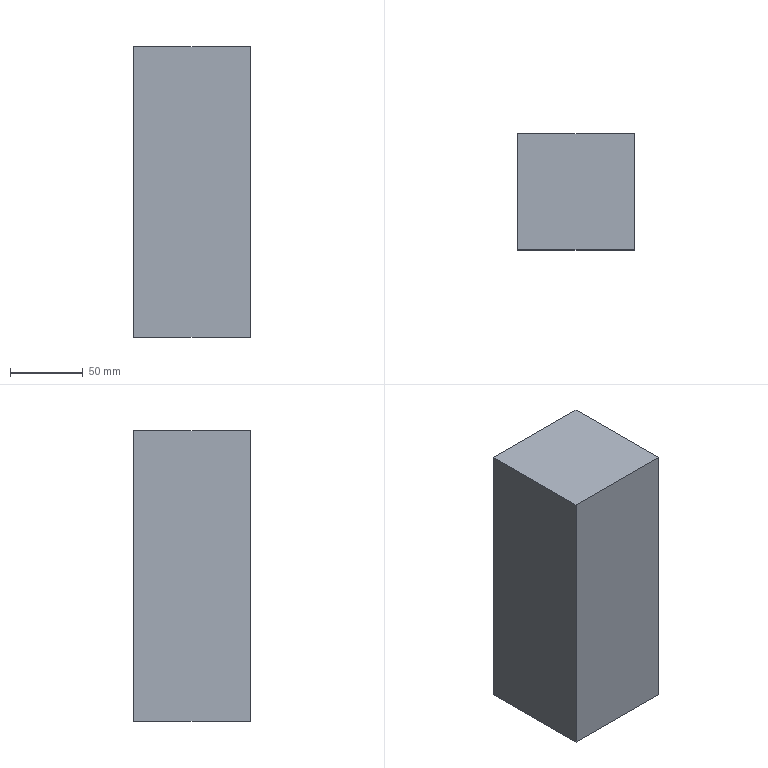Part | SolidWorks | features Extrusion 1 | 1 solid | 6 faces | box 80 x 80 x 200 mm | volume 1280000 mm3 | plane 6
STEP:
#1=CARTESIAN_POINT('',(40.,-40.,-100.));
#2=VERTEX_POINT('',#1);
#3=CARTESIAN_POINT('',(40.,40.,-100.));
#4=VERTEX_POINT('',#3);
#5=CARTESIAN_POINT('',(40.,40.,-100.));
#6=DIRECTION('',(0.,1.,0.));
#7=VECTOR('',#6,1000.);
#8=LINE('',#5,#7);
#9=EDGE_CURVE('',#2,#4,#8,.T.);
#10=ORIENTED_EDGE('',*,*,#9,.T.);
#11=CARTESIAN_POINT('',(40.,40.,100.));
#12=VERTEX_POINT('',#11);
#13=CARTESIAN_POINT('',(40.,40.,100.));
#14=DIRECTION('',(0.,0.,-1.));
#15=VECTOR('',#14,1000.);
#16=LINE('',#13,#15);
#17=EDGE_CURVE('',#12,#4,#16,.T.);
#18=ORIENTED_EDGE('',*,*,#17,.F.);
#19=CARTESIAN_POINT('',(40.,-40.,100.));
#20=VERTEX_POINT('',#19);
#21=CARTESIAN_POINT('',(40.,40.,100.));
#22=DIRECTION('',(0.,1.,0.));
#23=VECTOR('',#22,1000.);
#24=LINE('',#21,#23);
#25=EDGE_CURVE('',#20,#12,#24,.T.);
#26=ORIENTED_EDGE('',*,*,#25,.F.);
#27=CARTESIAN_POINT('',(40.,-40.,100.));
#28=DIRECTION('',(0.,0.,-1.));
#29=VECTOR('',#28,1000.);
#30=LINE('',#27,#29);
#31=EDGE_CURVE('',#20,#2,#30,.T.);
#32=ORIENTED_EDGE('',*,*,#31,.T.);
#33=EDGE_LOOP('',(#10,#18,#26,#32));
#34=FACE_OUTER_BOUND('',#33,.T.);
#35=CARTESIAN_POINT('',(40.,40.,100.));
#36=DIRECTION('',(-1.,0.,0.));
#37=DIRECTION('',(0.,-1.,0.));
#38=AXIS2_PLACEMENT_3D('',#35,#36,#37);
#39=PLANE('',#38);
#40=ADVANCED_FACE('',(#34),#39,.F.);
#41=CARTESIAN_POINT('',(-40.,40.,-100.));
#42=VERTEX_POINT('',#41);
#43=CARTESIAN_POINT('',(-40.,40.,-100.));
#44=DIRECTION('',(-1.,0.,0.));
#45=VECTOR('',#44,1000.);
#46=LINE('',#43,#45);
#47=EDGE_CURVE('',#4,#42,#46,.T.);
#48=ORIENTED_EDGE('',*,*,#47,.T.);
#49=CARTESIAN_POINT('',(-40.,40.,100.));
#50=VERTEX_POINT('',#49);
#51=CARTESIAN_POINT('',(-40.,40.,100.));
#52=DIRECTION('',(0.,0.,-1.));
#53=VECTOR('',#52,1000.);
#54=LINE('',#51,#53);
#55=EDGE_CURVE('',#50,#42,#54,.T.);
#56=ORIENTED_EDGE('',*,*,#55,.F.);
#57=CARTESIAN_POINT('',(-40.,40.,100.));
#58=DIRECTION('',(-1.,0.,0.));
#59=VECTOR('',#58,1000.);
#60=LINE('',#57,#59);
#61=EDGE_CURVE('',#12,#50,#60,.T.);
#62=ORIENTED_EDGE('',*,*,#61,.F.);
#63=ORIENTED_EDGE('',*,*,#17,.T.);
#64=EDGE_LOOP('',(#48,#56,#62,#63));
#65=FACE_OUTER_BOUND('',#64,.T.);
#66=CARTESIAN_POINT('',(-40.,40.,100.));
#67=DIRECTION('',(0.,-1.,0.));
#68=DIRECTION('',(0.,0.,-1.));
#69=AXIS2_PLACEMENT_3D('',#66,#67,#68);
#70=PLANE('',#69);
#71=ADVANCED_FACE('',(#65),#70,.F.);
#72=CARTESIAN_POINT('',(-40.,-40.,-100.));
#73=VERTEX_POINT('',#72);
#74=CARTESIAN_POINT('',(-40.,40.,-100.));
#75=DIRECTION('',(0.,-1.,0.));
#76=VECTOR('',#75,1000.);
#77=LINE('',#74,#76);
#78=EDGE_CURVE('',#42,#73,#77,.T.);
#79=ORIENTED_EDGE('',*,*,#78,.T.);
#80=CARTESIAN_POINT('',(-40.,-40.,100.));
#81=VERTEX_POINT('',#80);
#82=CARTESIAN_POINT('',(-40.,-40.,100.));
#83=DIRECTION('',(0.,0.,-1.));
#84=VECTOR('',#83,1000.);
#85=LINE('',#82,#84);
#86=EDGE_CURVE('',#81,#73,#85,.T.);
#87=ORIENTED_EDGE('',*,*,#86,.F.);
#88=CARTESIAN_POINT('',(-40.,40.,100.));
#89=DIRECTION('',(0.,-1.,0.));
#90=VECTOR('',#89,1000.);
#91=LINE('',#88,#90);
#92=EDGE_CURVE('',#50,#81,#91,.T.);
#93=ORIENTED_EDGE('',*,*,#92,.F.);
#94=ORIENTED_EDGE('',*,*,#55,.T.);
#95=EDGE_LOOP('',(#79,#87,#93,#94));
#96=FACE_OUTER_BOUND('',#95,.T.);
#97=CARTESIAN_POINT('',(-40.,40.,100.));
#98=DIRECTION('',(1.,0.,0.));
#99=DIRECTION('',(0.,0.,-1.));
#100=AXIS2_PLACEMENT_3D('',#97,#98,#99);
#101=PLANE('',#100);
#102=ADVANCED_FACE('',(#96),#101,.F.);
#103=CARTESIAN_POINT('',(-40.,-40.,-100.));
#104=DIRECTION('',(1.,0.,0.));
#105=VECTOR('',#104,1000.);
#106=LINE('',#103,#105);
#107=EDGE_CURVE('',#73,#2,#106,.T.);
#108=ORIENTED_EDGE('',*,*,#107,.T.);
#109=ORIENTED_EDGE('',*,*,#31,.F.);
#110=CARTESIAN_POINT('',(-40.,-40.,100.));
#111=DIRECTION('',(1.,0.,0.));
#112=VECTOR('',#111,1000.);
#113=LINE('',#110,#112);
#114=EDGE_CURVE('',#81,#20,#113,.T.);
#115=ORIENTED_EDGE('',*,*,#114,.F.);
#116=ORIENTED_EDGE('',*,*,#86,.T.);
#117=EDGE_LOOP('',(#108,#109,#115,#116));
#118=FACE_OUTER_BOUND('',#117,.T.);
#119=CARTESIAN_POINT('',(-40.,-40.,100.));
#120=DIRECTION('',(0.,1.,0.));
#121=DIRECTION('',(0.,0.,1.));
#122=AXIS2_PLACEMENT_3D('',#119,#120,#121);
#123=PLANE('',#122);
#124=ADVANCED_FACE('',(#118),#123,.F.);
#125=ORIENTED_EDGE('',*,*,#25,.T.);
#126=ORIENTED_EDGE('',*,*,#61,.T.);
#127=ORIENTED_EDGE('',*,*,#92,.T.);
#128=ORIENTED_EDGE('',*,*,#114,.T.);
#129=EDGE_LOOP('',(#125,#126,#127,#128));
#130=FACE_OUTER_BOUND('',#129,.T.);
#131=CARTESIAN_POINT('',(0.,0.,100.));
#132=DIRECTION('',(0.,0.,1.));
#133=DIRECTION('',(1.,0.,0.));
#134=AXIS2_PLACEMENT_3D('',#131,#132,#133);
#135=PLANE('',#134);
#136=ADVANCED_FACE('',(#130),#135,.T.);
#137=ORIENTED_EDGE('',*,*,#9,.F.);
#138=ORIENTED_EDGE('',*,*,#107,.F.);
#139=ORIENTED_EDGE('',*,*,#78,.F.);
#140=ORIENTED_EDGE('',*,*,#47,.F.);
#141=EDGE_LOOP('',(#137,#138,#139,#140));
#142=FACE_OUTER_BOUND('',#141,.T.);
#143=CARTESIAN_POINT('',(0.,0.,-100.));
#144=DIRECTION('',(0.,0.,1.));
#145=DIRECTION('',(1.,0.,0.));
#146=AXIS2_PLACEMENT_3D('',#143,#144,#145);
#147=PLANE('',#146);
#148=ADVANCED_FACE('',(#142),#147,.F.);
#149=CLOSED_SHELL('',(#40,#71,#102,#124,#136,#148));
#150=MANIFOLD_SOLID_BREP('',#149);
#151=CARTESIAN_POINT('',(0.,0.,0.));
#152=DIRECTION('',(0.,0.,1.));
#153=DIRECTION('',(1.,0.,0.));
#154=AXIS2_PLACEMENT_3D('',#151,#152,#153);
#155=(LENGTH_UNIT()NAMED_UNIT(*)SI_UNIT(.MILLI.,.METRE.));
#156=UNCERTAINTY_MEASURE_WITH_UNIT(LENGTH_MEASURE(0.00001),#155,'','');
#157=(NAMED_UNIT(*)PLANE_ANGLE_UNIT()SI_UNIT($,.RADIAN.));
#158=(NAMED_UNIT(*)SI_UNIT($,.STERADIAN.)SOLID_ANGLE_UNIT());
#159=(GEOMETRIC_REPRESENTATION_CONTEXT(3)GLOBAL_UNCERTAINTY_ASSIGNED_CONTEXT((#156))GLOBAL_UNIT_ASSIGNED_CONTEXT((#155,#157,#158))REPRESENTATION_CONTEXT('',''));
#160=ADVANCED_BREP_SHAPE_REPRESENTATION('',(#150,#154),#159);